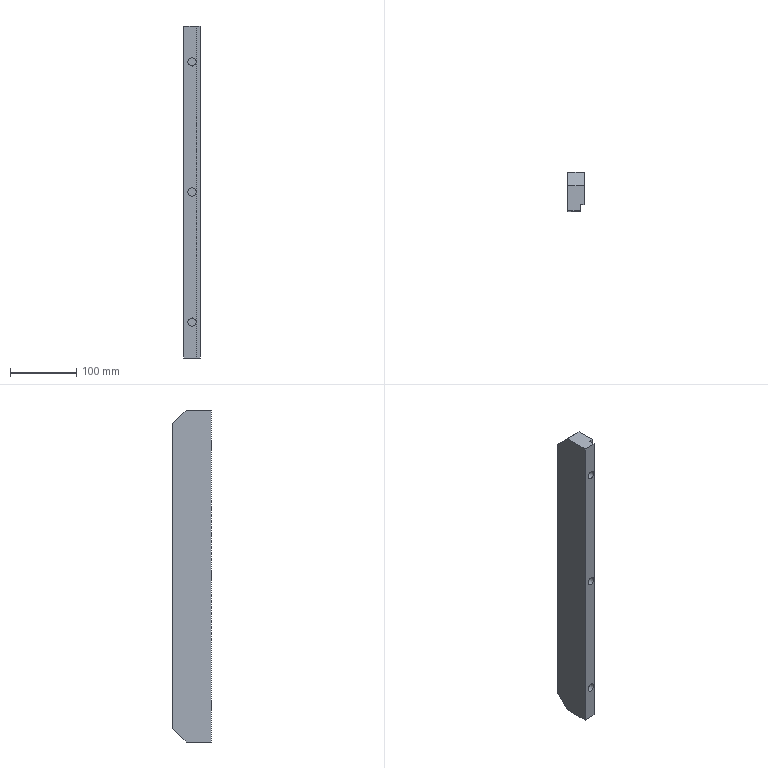NC program | NX | posted with a generic post | part box 25 x 58 x 500 mm
Whole program:
N10 G17 G21 G94 G90
(FLOOR_WALL , TOOL : D26R0.8)
N12 T02 M6
N14 G54
N16 G17 G0 G90 X-266. Y3. S1500 M3
N18 G43 Z30. H2
N20 Z7.667
N22 G94 G1 Z4.667 F2000.
N24 X-263.
N26 X263.
N28 X266.
N30 Z7.667
N32 G0 Z30.
N34 X-266.
N36 Z7.333
N38 G1 Z4.333
N40 X-263.
N42 X263.
N44 X266.
N46 Z7.333
N48 G0 Z30.
N50 X-266.
N52 Z7.
N54 G1 Z4.
N56 X-263.
N58 X263.
N60 X266.
N62 Z7.
N64 G0 Z30.
N66 X-266.
N68 Z6.667
N70 G1 Z3.667
N72 X-263.
N74 X263.
N76 X266.
N78 Z6.667
N80 G0 Z30.
N82 X-266.
N84 Z6.333
N86 G1 Z3.333
N88 X-263.
N90 X263.
N92 X266.
N94 Z6.333
N96 G0 Z30.
N98 X-266.
N100 Z6.
N102 G1 Z3.
N104 X-263.
N106 X263.
N108 X266.
N110 Z6.
N112 G0 Z30.
N114 X-266.
N116 Z5.667
N118 G1 Z2.667
N120 X-263.
N122 X263.
N124 X266.
N126 Z5.667
N128 G0 Z30.
N130 X-266.
N132 Z5.333
N134 G1 Z2.333
N136 X-263.
N138 X263.
N140 X266.
N142 Z5.333
N144 G0 Z30.
N146 X-266.
N148 Z5.
N150 G1 Z2.
N152 X-263.
N154 X263.
N156 X266.
N158 Z5.
N160 G0 Z30.
N162 X-266.
N164 Z4.667
N166 G1 Z1.667
N168 X-263.
N170 X263.
N172 X266.
N174 Z4.667
N176 G0 Z30.
N178 X-266.
N180 Z4.333
N182 G1 Z1.333
N184 X-263.
N186 X263.
N188 X266.
N190 Z4.333
N192 G0 Z30.
N194 X-266.
N196 Z4.
N198 G1 Z1.
N200 X-263.
N202 X263.
N204 X266.
N206 Z4.
N208 G0 Z30.
N210 X-266.
N212 Z3.667
N214 G1 Z0.667
N216 X-263.
N218 X263.
N220 X266.
N222 Z3.667
N224 G0 Z30.
N226 X-266.
N228 Z3.333
N230 G1 Z0.333
N232 X-263.
N234 X263.
N236 X266.
N238 Z3.333
N240 G0 Z30.
N242 X-266.
N244 Z3.
N246 G1 Z0.
N248 X-263.
N250 X263.
N252 X266.
N254 Z3.
N256 G0 Z30.
(ZLEVEL_PROFILE , TOOL : D26R0.8)
N258 X268.613 Y-24.284 S1800
N260 Z-5.291
N262 G1 X266.462 Y-20.825 F2200.
N264 G3 X264.169 Y-19.599 R2.6
N266 G1 X264.072 Y-19.602
N268 X250. Y-19.6
N270 X-249.089
N272 X-264.072 Y-19.602
N274 X-264.169 Y-19.599
N276 G3 X-266.462 Y-20.825 R2.6
N278 G1 X-268.612 Y-24.284
N280 G0 X-268.614 Y-24.283 Z-5.582
N282 G1 X-266.463 Y-20.825
N284 G2 X-264.17 Y-19.599 R2.6
N286 G1 X-264.072 Y-19.602
N288 X-249.089 Y-19.6
N290 X250.
N292 X264.072 Y-19.602
N294 X264.171 Y-19.599
N296 G2 X266.464 Y-20.825 R2.6
N298 G1 X268.614 Y-24.283
N300 G0 X268.615 Z-5.874
N302 G1 X266.465 Y-20.824
N304 G3 X264.172 Y-19.599 R2.6
N306 G1 X264.072 Y-19.602
N308 X250. Y-19.6
N310 X-249.089
N312 X-264.072 Y-19.602
N314 X-264.172 Y-19.599
N316 G3 X-266.465 Y-20.824 R2.6
N318 G1 X-268.615 Y-24.283
N320 G0 X-268.617 Z-6.165
N322 G1 X-266.466 Y-20.824
N324 G2 X-264.173 Y-19.599 R2.6
N326 G1 X-264.072 Y-19.602
N328 X-249.089 Y-19.6
N330 X250.
N332 X264.072 Y-19.602
N334 X264.174 Y-19.599
N336 G2 X266.467 Y-20.824 R2.6
N338 G1 X268.617 Y-24.283
N340 G0 X268.618 Y-24.282 Z-6.456
N342 G1 X266.468 Y-20.824
N344 G3 X264.175 Y-19.599 R2.6
N346 G1 X264.072 Y-19.602
N348 X250. Y-19.6
N350 X-249.089
N352 X-264.072 Y-19.602
N354 X-264.175 Y-19.599
N356 G3 X-266.468 Y-20.824 R2.6
N358 G1 X-268.618 Y-24.282
N360 G0 X-268.619 Z-6.747
N362 G1 X-266.469 Y-20.824
N364 G2 X-264.176 Y-19.599 R2.6
N366 G1 X-264.072 Y-19.602
N368 X-249.089 Y-19.6
N370 X250.
N372 X264.072 Y-19.602
N374 X264.177 Y-19.599
N376 G2 X266.47 Y-20.824 R2.6
N378 G1 X268.619 Y-24.282
N380 G0 X268.621 Z-7.038
N382 G1 X266.471 Y-20.824
N384 G3 X264.178 Y-19.599 R2.6
N386 G1 X264.072 Y-19.602
N388 X250. Y-19.6
N390 X-249.089
N392 X-264.072 Y-19.602
N394 X-264.178 Y-19.599
N396 G3 X-266.471 Y-20.824 R2.6
N398 G1 X-268.621 Y-24.282
N400 G0 X-268.622 Y-24.281 Z-7.329
N402 G1 X-266.472 Y-20.824
N404 G2 X-264.179 Y-19.599 R2.6
N406 G1 X-264.072 Y-19.602
N408 X-249.089 Y-19.6
N410 X250.
N412 X264.072 Y-19.602
N414 X264.18 Y-19.599
N416 G2 X266.473 Y-20.824 R2.6
N418 G1 X268.622 Y-24.281
N420 G0 X268.624 Z-7.621
N422 G1 X266.474 Y-20.824
N424 G3 X264.181 Y-19.598 R2.6
N426 G1 X264.072 Y-19.602
N428 X251.274
N430 X250. Y-19.6
N432 X-249.089
N434 X-264.072 Y-19.602
N436 X-264.181 Y-19.599
N438 G3 X-266.474 Y-20.824 R2.6
N440 G1 X-268.623 Y-24.281
N442 G0 X-268.625 Z-7.912
N444 G1 X-266.475 Y-20.824
N446 G2 X-264.182 Y-19.598 R2.6
N448 G1 X-264.072 Y-19.602
N450 X-249.089 Y-19.6
N452 X250.
N454 X251.274 Y-19.602
N456 X264.072
N458 X264.183 Y-19.598
N460 G2 X266.476 Y-20.824 R2.6
N462 G1 X268.625 Y-24.281
N464 G0 X268.626 Y-24.28 Z-8.203
N466 G1 X266.477 Y-20.824
N468 G3 X264.184 Y-19.598 R2.6
N470 G1 X264.072 Y-19.602
N472 X251.274
N474 X250. Y-19.6
N476 X-249.089
N478 X-264.072 Y-19.602
N480 X-264.184 Y-19.598
N482 G3 X-266.477 Y-20.824 R2.6
N484 G1 X-268.626 Y-24.28
N486 G0 X-268.627 Z-8.494
N488 G1 X-266.478 Y-20.824
N490 G2 X-264.185 Y-19.598 R2.6
N492 G1 X-264.072 Y-19.602
N494 X-249.089 Y-19.6
N496 X250.
N498 X251.274 Y-19.602
N500 X264.072
N502 X264.186 Y-19.598
N504 G2 X266.479 Y-20.824 R2.6
N506 G1 X268.628 Y-24.28
N508 G0 X268.629 Y-24.279 Z-8.785
N510 G1 X266.48 Y-20.824
N512 G3 X264.187 Y-19.598 R2.6
N514 G1 X264.072 Y-19.602
N516 X251.274
N518 X250. Y-19.6
N520 X-249.089
N522 X-264.072 Y-19.602
N524 X-264.187 Y-19.598
N526 G3 X-266.48 Y-20.824 R2.6
N528 G1 X-268.629 Y-24.279
N530 G0 X-268.63 Z-9.076
N532 G1 X-266.481 Y-20.824
N534 G2 X-264.188 Y-19.598 R2.6
N536 G1 X-264.072 Y-19.602
N538 X-249.089 Y-19.6
N540 X250.
N542 X251.274 Y-19.602
N544 X264.072
N546 X264.189 Y-19.598
N548 G2 X266.482 Y-20.824 R2.6
N550 G1 X268.63 Y-24.279
N552 G0 X268.632 Z-9.368
N554 G1 X266.483 Y-20.824
N556 G3 X264.19 Y-19.598 R2.6
N558 G1 X264.072 Y-19.602
N560 X251.274
N562 X250. Y-19.6
N564 X-249.089
N566 X-264.072 Y-19.602
N568 X-264.19 Y-19.598
N570 G3 X-266.483 Y-20.824 R2.6
N572 G1 X-268.632 Y-24.279
N574 G0 X-268.633 Y-24.278 Z-9.659
N576 G1 X-266.484 Y-20.824
N578 G2 X-264.191 Y-19.598 R2.6
N580 G1 X-264.072 Y-19.602
N582 X-249.089 Y-19.6
N584 X250.
N586 X251.274 Y-19.602
N588 X264.072
N590 X264.192 Y-19.598
N592 G2 X266.485 Y-20.824 R2.6
N594 G1 X268.633 Y-24.278
N596 G0 Z30.
N598 M5
(DRILLING_COPY , TOOL : 12.5ZT)
N600 T03 M6
N602 G54
N604 G17 G0 G90 X-196. Y0. S800 M3
N606 G43 Z30. H3
N608 G94 G83 G98 Z-36.755 F120. Q2. R3.
N610 X0.
N612 X196.
N614 G80
N616 G0 X196. Y0. Z30.
N618 M5
(FLOOR_WALL_1 , TOOL : D10JING)
N620 T11 M6
N622 G54
N624 G17 G0 G90 X258. Y-11.5 S5000 M3
N626 G43 Z30. H11
N628 Z-7.
N630 G94 G1 Z-10. F1250.
N632 X250.
N634 X-250.
N636 X-258.
N638 Z-7.
N640 G0 Z30.
N642 M5
(ZLEVEL_PROFILE_COPY_1_COPY_COPY_COPY_COPY , TOOL : D6A45)
N644 T07 M6
N646 G54
N648 G17 G0 G90 X251.951 Y-10.168 S7000 M3
N650 G43 Z30. H7
N652 Z-11.
N654 G94 G1 X251.34 Y-9.631 F1000.
N656 G3 X250.751 Y-9.514 R0.6
N658 G1 Y-12.501
N660 G2 X250.001 Y-13.251 R0.751
N662 G1 X-250.001
N664 G2 X-250.751 Y-12.501 R0.751
N666 G1 Y-9.514
N668 G3 X-251.34 Y-9.631 R0.6
N670 G1 X-251.951 Y-10.169
N672 G0 Z30.
N674 M5
N676 M2